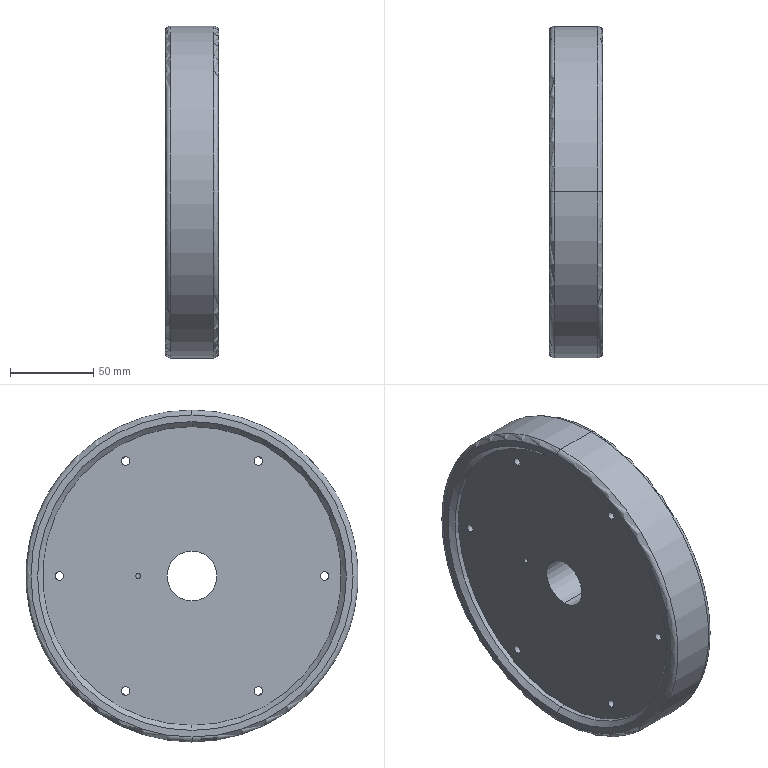Part | SolidWorks | features Fillet 2, 3DProfileFeature 1, Chamfer 1, CirPattern 1, HoleWzd 1, ICE 1, Revolution 1 | 1 solid | 46 faces | box 32 x 200 x 200 mm | volume 440952 mm3 | cylinder 20 | plane 12 | torus 8 | cone 6 | commonest cylinder face diameters 5 x12 3 x2 30 x2 180 x2 200 x2